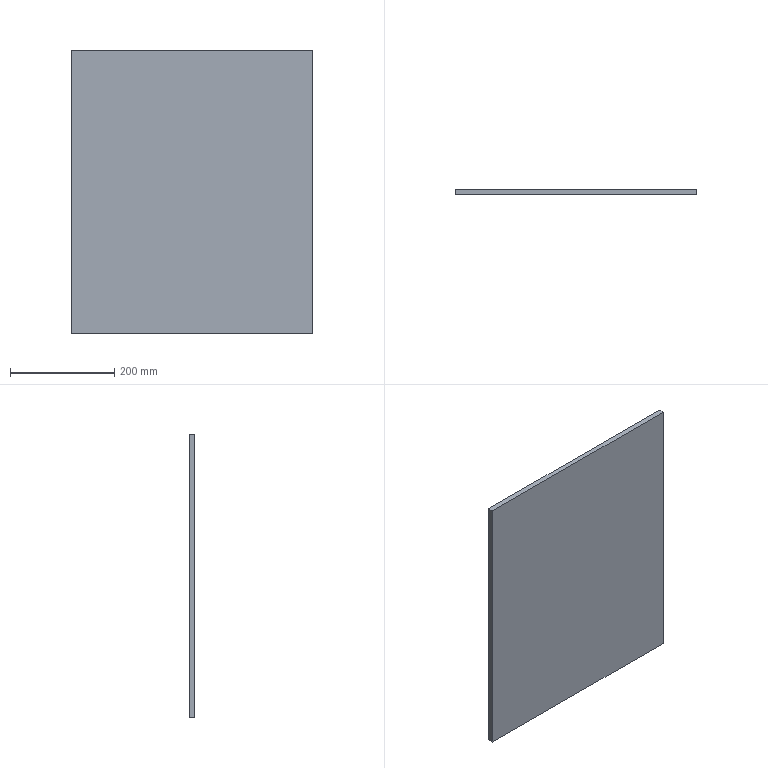Part | SolidWorks | features Extrusion 1 | 1 solid | 6 faces | box 463.2 x 10.2 x 543.2 mm | volume 2566424 mm3 | plane 6
STEP:
#1=CARTESIAN_POINT('',(0.,0.,-543.2));
#2=VERTEX_POINT('',#1);
#3=CARTESIAN_POINT('',(0.,0.,0.));
#4=VERTEX_POINT('',#3);
#5=CARTESIAN_POINT('',(0.,0.,0.));
#6=DIRECTION('',(0.,0.,1.));
#7=VECTOR('',#6,1000.);
#8=LINE('',#5,#7);
#9=EDGE_CURVE('',#2,#4,#8,.T.);
#10=ORIENTED_EDGE('',*,*,#9,.T.);
#11=CARTESIAN_POINT('',(0.,10.2,0.));
#12=VERTEX_POINT('',#11);
#13=CARTESIAN_POINT('',(0.,10.2,0.));
#14=DIRECTION('',(0.,-1.,0.));
#15=VECTOR('',#14,1000.);
#16=LINE('',#13,#15);
#17=EDGE_CURVE('',#12,#4,#16,.T.);
#18=ORIENTED_EDGE('',*,*,#17,.F.);
#19=CARTESIAN_POINT('',(0.,10.2,-543.2));
#20=VERTEX_POINT('',#19);
#21=CARTESIAN_POINT('',(0.,10.2,0.));
#22=DIRECTION('',(0.,0.,1.));
#23=VECTOR('',#22,1000.);
#24=LINE('',#21,#23);
#25=EDGE_CURVE('',#20,#12,#24,.T.);
#26=ORIENTED_EDGE('',*,*,#25,.F.);
#27=CARTESIAN_POINT('',(0.,10.2,-543.2));
#28=DIRECTION('',(0.,-1.,0.));
#29=VECTOR('',#28,1000.);
#30=LINE('',#27,#29);
#31=EDGE_CURVE('',#20,#2,#30,.T.);
#32=ORIENTED_EDGE('',*,*,#31,.T.);
#33=EDGE_LOOP('',(#10,#18,#26,#32));
#34=FACE_OUTER_BOUND('',#33,.T.);
#35=CARTESIAN_POINT('',(0.,10.2,0.));
#36=DIRECTION('',(1.,0.,0.));
#37=DIRECTION('',(0.,0.,-1.));
#38=AXIS2_PLACEMENT_3D('',#35,#36,#37);
#39=PLANE('',#38);
#40=ADVANCED_FACE('',(#34),#39,.F.);
#41=CARTESIAN_POINT('',(463.2,0.,0.));
#42=VERTEX_POINT('',#41);
#43=CARTESIAN_POINT('',(0.,0.,0.));
#44=DIRECTION('',(1.,0.,0.));
#45=VECTOR('',#44,1000.);
#46=LINE('',#43,#45);
#47=EDGE_CURVE('',#4,#42,#46,.T.);
#48=ORIENTED_EDGE('',*,*,#47,.T.);
#49=CARTESIAN_POINT('',(463.2,10.2,0.));
#50=VERTEX_POINT('',#49);
#51=CARTESIAN_POINT('',(463.2,10.2,0.));
#52=DIRECTION('',(0.,-1.,0.));
#53=VECTOR('',#52,1000.);
#54=LINE('',#51,#53);
#55=EDGE_CURVE('',#50,#42,#54,.T.);
#56=ORIENTED_EDGE('',*,*,#55,.F.);
#57=CARTESIAN_POINT('',(0.,10.2,0.));
#58=DIRECTION('',(1.,0.,0.));
#59=VECTOR('',#58,1000.);
#60=LINE('',#57,#59);
#61=EDGE_CURVE('',#12,#50,#60,.T.);
#62=ORIENTED_EDGE('',*,*,#61,.F.);
#63=ORIENTED_EDGE('',*,*,#17,.T.);
#64=EDGE_LOOP('',(#48,#56,#62,#63));
#65=FACE_OUTER_BOUND('',#64,.T.);
#66=CARTESIAN_POINT('',(0.,10.2,0.));
#67=DIRECTION('',(0.,0.,-1.));
#68=DIRECTION('',(-1.,0.,0.));
#69=AXIS2_PLACEMENT_3D('',#66,#67,#68);
#70=PLANE('',#69);
#71=ADVANCED_FACE('',(#65),#70,.F.);
#72=CARTESIAN_POINT('',(463.2,0.,-543.2));
#73=VERTEX_POINT('',#72);
#74=CARTESIAN_POINT('',(463.2,0.,0.));
#75=DIRECTION('',(0.,0.,-1.));
#76=VECTOR('',#75,1000.);
#77=LINE('',#74,#76);
#78=EDGE_CURVE('',#42,#73,#77,.T.);
#79=ORIENTED_EDGE('',*,*,#78,.T.);
#80=CARTESIAN_POINT('',(463.2,10.2,-543.2));
#81=VERTEX_POINT('',#80);
#82=CARTESIAN_POINT('',(463.2,10.2,-543.2));
#83=DIRECTION('',(0.,-1.,0.));
#84=VECTOR('',#83,1000.);
#85=LINE('',#82,#84);
#86=EDGE_CURVE('',#81,#73,#85,.T.);
#87=ORIENTED_EDGE('',*,*,#86,.F.);
#88=CARTESIAN_POINT('',(463.2,10.2,0.));
#89=DIRECTION('',(0.,0.,-1.));
#90=VECTOR('',#89,1000.);
#91=LINE('',#88,#90);
#92=EDGE_CURVE('',#50,#81,#91,.T.);
#93=ORIENTED_EDGE('',*,*,#92,.F.);
#94=ORIENTED_EDGE('',*,*,#55,.T.);
#95=EDGE_LOOP('',(#79,#87,#93,#94));
#96=FACE_OUTER_BOUND('',#95,.T.);
#97=CARTESIAN_POINT('',(463.2,10.2,0.));
#98=DIRECTION('',(-1.,0.,0.));
#99=DIRECTION('',(0.,0.,1.));
#100=AXIS2_PLACEMENT_3D('',#97,#98,#99);
#101=PLANE('',#100);
#102=ADVANCED_FACE('',(#96),#101,.F.);
#103=CARTESIAN_POINT('',(0.,0.,-543.2));
#104=DIRECTION('',(-1.,0.,0.));
#105=VECTOR('',#104,1000.);
#106=LINE('',#103,#105);
#107=EDGE_CURVE('',#73,#2,#106,.T.);
#108=ORIENTED_EDGE('',*,*,#107,.T.);
#109=ORIENTED_EDGE('',*,*,#31,.F.);
#110=CARTESIAN_POINT('',(0.,10.2,-543.2));
#111=DIRECTION('',(-1.,0.,0.));
#112=VECTOR('',#111,1000.);
#113=LINE('',#110,#112);
#114=EDGE_CURVE('',#81,#20,#113,.T.);
#115=ORIENTED_EDGE('',*,*,#114,.F.);
#116=ORIENTED_EDGE('',*,*,#86,.T.);
#117=EDGE_LOOP('',(#108,#109,#115,#116));
#118=FACE_OUTER_BOUND('',#117,.T.);
#119=CARTESIAN_POINT('',(0.,10.2,-543.2));
#120=DIRECTION('',(0.,0.,1.));
#121=DIRECTION('',(1.,0.,0.));
#122=AXIS2_PLACEMENT_3D('',#119,#120,#121);
#123=PLANE('',#122);
#124=ADVANCED_FACE('',(#118),#123,.F.);
#125=ORIENTED_EDGE('',*,*,#25,.T.);
#126=ORIENTED_EDGE('',*,*,#61,.T.);
#127=ORIENTED_EDGE('',*,*,#92,.T.);
#128=ORIENTED_EDGE('',*,*,#114,.T.);
#129=EDGE_LOOP('',(#125,#126,#127,#128));
#130=FACE_OUTER_BOUND('',#129,.T.);
#131=CARTESIAN_POINT('',(0.,10.2,0.));
#132=DIRECTION('',(0.,-1.,0.));
#133=DIRECTION('',(0.,0.,-1.));
#134=AXIS2_PLACEMENT_3D('',#131,#132,#133);
#135=PLANE('',#134);
#136=ADVANCED_FACE('',(#130),#135,.F.);
#137=ORIENTED_EDGE('',*,*,#9,.F.);
#138=ORIENTED_EDGE('',*,*,#107,.F.);
#139=ORIENTED_EDGE('',*,*,#78,.F.);
#140=ORIENTED_EDGE('',*,*,#47,.F.);
#141=EDGE_LOOP('',(#137,#138,#139,#140));
#142=FACE_OUTER_BOUND('',#141,.T.);
#143=CARTESIAN_POINT('',(0.,0.,0.));
#144=DIRECTION('',(0.,-1.,0.));
#145=DIRECTION('',(0.,0.,-1.));
#146=AXIS2_PLACEMENT_3D('',#143,#144,#145);
#147=PLANE('',#146);
#148=ADVANCED_FACE('',(#142),#147,.T.);
#149=CLOSED_SHELL('',(#40,#71,#102,#124,#136,#148));
#150=MANIFOLD_SOLID_BREP('',#149);
#151=CARTESIAN_POINT('',(0.,0.,0.));
#152=DIRECTION('',(0.,0.,1.));
#153=DIRECTION('',(1.,0.,0.));
#154=AXIS2_PLACEMENT_3D('',#151,#152,#153);
#155=(LENGTH_UNIT()NAMED_UNIT(*)SI_UNIT(.MILLI.,.METRE.));
#156=UNCERTAINTY_MEASURE_WITH_UNIT(LENGTH_MEASURE(0.00001),#155,'','');
#157=(NAMED_UNIT(*)PLANE_ANGLE_UNIT()SI_UNIT($,.RADIAN.));
#158=(NAMED_UNIT(*)SI_UNIT($,.STERADIAN.)SOLID_ANGLE_UNIT());
#159=(GEOMETRIC_REPRESENTATION_CONTEXT(3)GLOBAL_UNCERTAINTY_ASSIGNED_CONTEXT((#156))GLOBAL_UNIT_ASSIGNED_CONTEXT((#155,#157,#158))REPRESENTATION_CONTEXT('',''));
#160=ADVANCED_BREP_SHAPE_REPRESENTATION('',(#150,#154),#159);